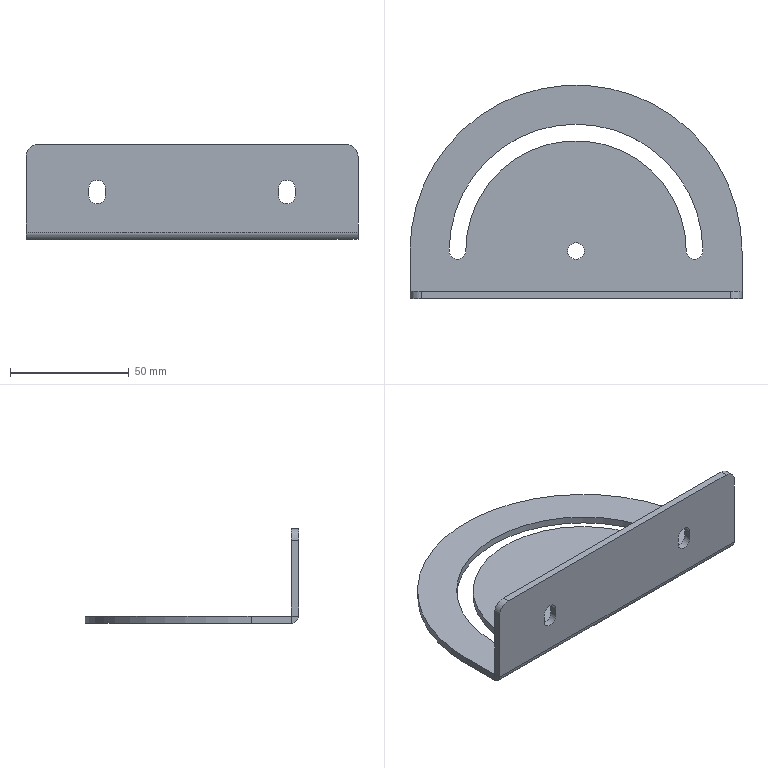Part | STEP file | Magazine bracket mounting plate | 1 solid | 32 faces | box 140 x 90 x 40 mm | volume 42824 mm3 | cylinder 17 | plane 15 | commonest cylinder face diameters 7 x10 10 x2 0.2 x1 6.2 x1 93 x1 107 x1